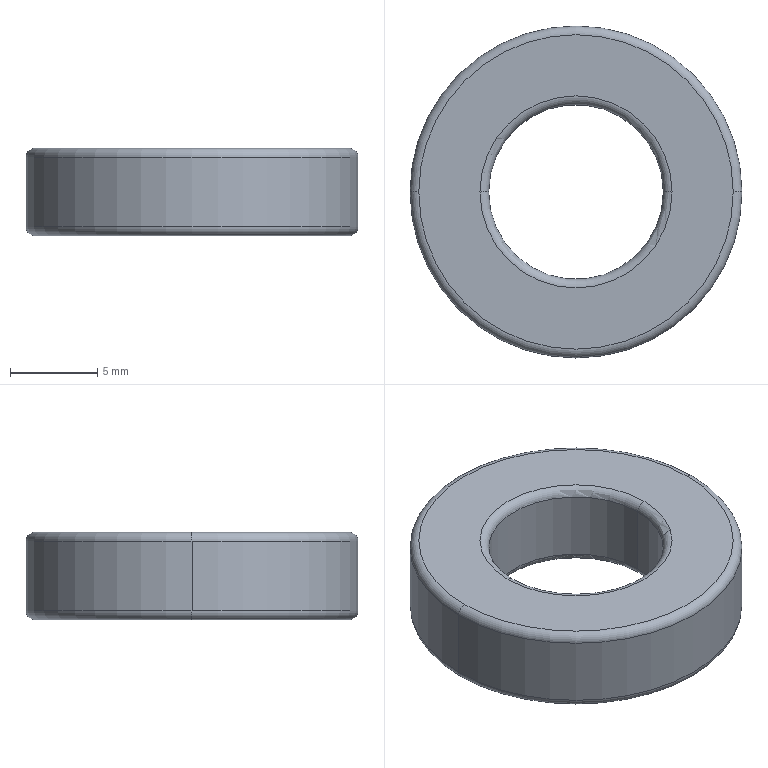Part | STEP file | 6800ZZ | 1 solid | 14 faces | box 19 x 19 x 5 mm | volume 1015 mm3 | torus 8 | cylinder 4 | plane 2 | commonest cylinder face diameters 10 x2 19 x2
STEP:
#1=CARTESIAN_POINT('',(0.,0.,0.));
#2=DIRECTION('',(0.,0.,1.));
#3=DIRECTION('',(1.,0.,0.));
#4=AXIS2_PLACEMENT_3D('',#1,#2,#3);
#5=CARTESIAN_POINT('',(-5.,0.,0.5));
#6=VERTEX_POINT('',#5);
#7=CARTESIAN_POINT('',(5.,0.,0.5));
#8=VERTEX_POINT('',#7);
#9=CARTESIAN_POINT('',(0.,0.,0.5));
#10=DIRECTION('',(0.,0.,-1.));
#11=DIRECTION('',(1.,0.,0.));
#12=AXIS2_PLACEMENT_3D('',#9,#10,#11);
#13=CIRCLE('',#12,5.);
#14=CARTESIAN_POINT('',(0.,0.,0.5));
#15=DIRECTION('',(0.,0.,1.));
#16=DIRECTION('',(1.,0.,0.));
#17=AXIS2_PLACEMENT_3D('',#14,#15,#16);
#18=TOROIDAL_SURFACE('',#17,5.5,0.5);
#19=CARTESIAN_POINT('',(6.283,3.142));
#20=DIRECTION('',(-1.,0.));
#21=VECTOR('',#20,1.);
#22=LINE('',#19,#21);
#23=(GEOMETRIC_REPRESENTATION_CONTEXT(2)PARAMETRIC_REPRESENTATION_CONTEXT()REPRESENTATION_CONTEXT('',''));
#24=DEFINITIONAL_REPRESENTATION('',(#22),#23);
#25=PCURVE('',#18,#24);
#26=CARTESIAN_POINT('',(0.,0.,5.));
#27=DIRECTION('',(0.,0.,-1.));
#28=DIRECTION('',(-1.,0.,0.));
#29=AXIS2_PLACEMENT_3D('',#26,#27,#28);
#30=CYLINDRICAL_SURFACE('',#29,5.);
#31=CARTESIAN_POINT('',(-3.142,4.5));
#32=DIRECTION('',(1.,0.));
#33=VECTOR('',#32,1.);
#34=LINE('',#31,#33);
#35=(GEOMETRIC_REPRESENTATION_CONTEXT(2)PARAMETRIC_REPRESENTATION_CONTEXT()REPRESENTATION_CONTEXT('',''));
#36=DEFINITIONAL_REPRESENTATION('',(#34),#35);
#37=PCURVE('',#30,#36);
#38=SURFACE_CURVE('',#13,(#25,#37),.PCURVE_S1.);
#39=EDGE_CURVE('',#6,#8,#38,.T.);
#40=ORIENTED_EDGE('',*,*,#39,.F.);
#41=CARTESIAN_POINT('',(-5.5,0.,0.));
#42=VERTEX_POINT('',#41);
#43=CARTESIAN_POINT('',(-5.5,0.,0.5));
#44=DIRECTION('',(0.,1.,0.));
#45=DIRECTION('',(-1.,0.,0.));
#46=AXIS2_PLACEMENT_3D('',#43,#44,#45);
#47=CIRCLE('',#46,0.5);
#48=CARTESIAN_POINT('',(3.142,0.));
#49=DIRECTION('',(0.,1.));
#50=VECTOR('',#49,1.);
#51=LINE('',#48,#50);
#52=(GEOMETRIC_REPRESENTATION_CONTEXT(2)PARAMETRIC_REPRESENTATION_CONTEXT()REPRESENTATION_CONTEXT('',''));
#53=DEFINITIONAL_REPRESENTATION('',(#51),#52);
#54=PCURVE('',#18,#53);
#55=CARTESIAN_POINT('',(0.,0.,0.5));
#56=DIRECTION('',(0.,0.,1.));
#57=DIRECTION('',(1.,0.,0.));
#58=AXIS2_PLACEMENT_3D('',#55,#56,#57);
#59=TOROIDAL_SURFACE('',#58,5.5,0.5);
#60=CARTESIAN_POINT('',(3.142,0.));
#61=DIRECTION('',(0.,1.));
#62=VECTOR('',#61,1.);
#63=LINE('',#60,#62);
#64=(GEOMETRIC_REPRESENTATION_CONTEXT(2)PARAMETRIC_REPRESENTATION_CONTEXT()REPRESENTATION_CONTEXT('',''));
#65=DEFINITIONAL_REPRESENTATION('',(#63),#64);
#66=PCURVE('',#59,#65);
#67=SURFACE_CURVE('',#47,(#54,#66),.PCURVE_S1.);
#68=EDGE_CURVE('',#6,#42,#67,.T.);
#69=ORIENTED_EDGE('',*,*,#68,.T.);
#70=CARTESIAN_POINT('',(5.5,0.,0.));
#71=VERTEX_POINT('',#70);
#72=CARTESIAN_POINT('',(0.,0.,0.));
#73=DIRECTION('',(0.,0.,1.));
#74=DIRECTION('',(1.,0.,0.));
#75=AXIS2_PLACEMENT_3D('',#72,#73,#74);
#76=CIRCLE('',#75,5.5);
#77=CARTESIAN_POINT('',(0.,4.712));
#78=DIRECTION('',(1.,0.));
#79=VECTOR('',#78,1.);
#80=LINE('',#77,#79);
#81=(GEOMETRIC_REPRESENTATION_CONTEXT(2)PARAMETRIC_REPRESENTATION_CONTEXT()REPRESENTATION_CONTEXT('',''));
#82=DEFINITIONAL_REPRESENTATION('',(#80),#81);
#83=PCURVE('',#18,#82);
#84=CARTESIAN_POINT('',(0.,0.,0.));
#85=DIRECTION('',(0.,0.,1.));
#86=DIRECTION('',(1.,0.,0.));
#87=AXIS2_PLACEMENT_3D('',#84,#85,#86);
#88=PLANE('',#87);
#89=CARTESIAN_POINT('',(0.,0.));
#90=DIRECTION('',(1.,0.));
#91=AXIS2_PLACEMENT_2D('',#89,#90);
#92=CIRCLE('',#91,5.5);
#93=(GEOMETRIC_REPRESENTATION_CONTEXT(2)PARAMETRIC_REPRESENTATION_CONTEXT()REPRESENTATION_CONTEXT('',''));
#94=DEFINITIONAL_REPRESENTATION('',(#92),#93);
#95=PCURVE('',#88,#94);
#96=SURFACE_CURVE('',#76,(#83,#95),.PCURVE_S1.);
#97=EDGE_CURVE('',#71,#42,#96,.T.);
#98=ORIENTED_EDGE('',*,*,#97,.F.);
#99=CARTESIAN_POINT('',(5.5,0.,0.5));
#100=DIRECTION('',(0.,-1.,0.));
#101=DIRECTION('',(0.,0.,-1.));
#102=AXIS2_PLACEMENT_3D('',#99,#100,#101);
#103=CIRCLE('',#102,0.5);
#104=CARTESIAN_POINT('',(0.,-1.571));
#105=DIRECTION('',(0.,1.));
#106=VECTOR('',#105,1.);
#107=LINE('',#104,#106);
#108=(GEOMETRIC_REPRESENTATION_CONTEXT(2)PARAMETRIC_REPRESENTATION_CONTEXT()REPRESENTATION_CONTEXT('',''));
#109=DEFINITIONAL_REPRESENTATION('',(#107),#108);
#110=PCURVE('',#18,#109);
#111=CARTESIAN_POINT('',(6.283,-1.571));
#112=DIRECTION('',(0.,1.));
#113=VECTOR('',#112,1.);
#114=LINE('',#111,#113);
#115=(GEOMETRIC_REPRESENTATION_CONTEXT(2)PARAMETRIC_REPRESENTATION_CONTEXT()REPRESENTATION_CONTEXT('',''));
#116=DEFINITIONAL_REPRESENTATION('',(#114),#115);
#117=PCURVE('',#59,#116);
#118=SURFACE_CURVE('',#103,(#110,#117),.PCURVE_S1.);
#119=EDGE_CURVE('',#8,#71,#118,.T.);
#120=ORIENTED_EDGE('',*,*,#119,.F.);
#121=EDGE_LOOP('',(#40,#69,#98,#120));
#122=FACE_BOUND('',#121,.T.);
#123=ADVANCED_FACE('',(#122),#18,.T.);
#124=CARTESIAN_POINT('',(-5.5,0.,5.));
#125=VERTEX_POINT('',#124);
#126=CARTESIAN_POINT('',(5.5,0.,5.));
#127=VERTEX_POINT('',#126);
#128=CARTESIAN_POINT('',(0.,0.,5.));
#129=DIRECTION('',(0.,0.,-1.));
#130=DIRECTION('',(1.,0.,0.));
#131=AXIS2_PLACEMENT_3D('',#128,#129,#130);
#132=CIRCLE('',#131,5.5);
#133=CARTESIAN_POINT('',(0.,0.,4.5));
#134=DIRECTION('',(0.,0.,1.));
#135=DIRECTION('',(1.,0.,0.));
#136=AXIS2_PLACEMENT_3D('',#133,#134,#135);
#137=TOROIDAL_SURFACE('',#136,5.5,0.5);
#138=CARTESIAN_POINT('',(6.283,1.571));
#139=DIRECTION('',(-1.,0.));
#140=VECTOR('',#139,1.);
#141=LINE('',#138,#140);
#142=(GEOMETRIC_REPRESENTATION_CONTEXT(2)PARAMETRIC_REPRESENTATION_CONTEXT()REPRESENTATION_CONTEXT('',''));
#143=DEFINITIONAL_REPRESENTATION('',(#141),#142);
#144=PCURVE('',#137,#143);
#145=CARTESIAN_POINT('',(0.,0.,5.));
#146=DIRECTION('',(0.,0.,1.));
#147=DIRECTION('',(1.,0.,0.));
#148=AXIS2_PLACEMENT_3D('',#145,#146,#147);
#149=PLANE('',#148);
#150=CARTESIAN_POINT('',(5.5,0.));
#151=CARTESIAN_POINT('',(5.5,-9.526));
#152=CARTESIAN_POINT('',(-2.75,-4.763));
#153=CARTESIAN_POINT('',(-11.,0.));
#154=CARTESIAN_POINT('',(-2.75,4.763));
#155=CARTESIAN_POINT('',(5.5,9.526));
#156=CARTESIAN_POINT('',(5.5,0.));
#157=(BOUNDED_CURVE()B_SPLINE_CURVE(2,(#150,#151,#152,#153,#154,#155,#156),.UNSPECIFIED.,.T.,.F.)B_SPLINE_CURVE_WITH_KNOTS((1,2,2,2,2,1),(-2.094,0.,2.094,4.189,6.283,8.378),.UNSPECIFIED.)CURVE()GEOMETRIC_REPRESENTATION_ITEM()RATIONAL_B_SPLINE_CURVE((1.,0.5,1.,0.5,1.,0.5,1.))REPRESENTATION_ITEM(''));
#158=(GEOMETRIC_REPRESENTATION_CONTEXT(2)PARAMETRIC_REPRESENTATION_CONTEXT()REPRESENTATION_CONTEXT('',''));
#159=DEFINITIONAL_REPRESENTATION('',(#157),#158);
#160=PCURVE('',#149,#159);
#161=SURFACE_CURVE('',#132,(#144,#160),.PCURVE_S1.);
#162=EDGE_CURVE('',#125,#127,#161,.T.);
#163=ORIENTED_EDGE('',*,*,#162,.F.);
#164=CARTESIAN_POINT('',(-5.,0.,4.5));
#165=VERTEX_POINT('',#164);
#166=CARTESIAN_POINT('',(-5.5,0.,4.5));
#167=DIRECTION('',(0.,1.,0.));
#168=DIRECTION('',(-1.,0.,0.));
#169=AXIS2_PLACEMENT_3D('',#166,#167,#168);
#170=CIRCLE('',#169,0.5);
#171=CARTESIAN_POINT('',(3.142,0.));
#172=DIRECTION('',(0.,1.));
#173=VECTOR('',#172,1.);
#174=LINE('',#171,#173);
#175=(GEOMETRIC_REPRESENTATION_CONTEXT(2)PARAMETRIC_REPRESENTATION_CONTEXT()REPRESENTATION_CONTEXT('',''));
#176=DEFINITIONAL_REPRESENTATION('',(#174),#175);
#177=PCURVE('',#137,#176);
#178=CARTESIAN_POINT('',(0.,0.,4.5));
#179=DIRECTION('',(0.,0.,1.));
#180=DIRECTION('',(1.,0.,0.));
#181=AXIS2_PLACEMENT_3D('',#178,#179,#180);
#182=TOROIDAL_SURFACE('',#181,5.5,0.5);
#183=CARTESIAN_POINT('',(3.142,0.));
#184=DIRECTION('',(0.,1.));
#185=VECTOR('',#184,1.);
#186=LINE('',#183,#185);
#187=(GEOMETRIC_REPRESENTATION_CONTEXT(2)PARAMETRIC_REPRESENTATION_CONTEXT()REPRESENTATION_CONTEXT('',''));
#188=DEFINITIONAL_REPRESENTATION('',(#186),#187);
#189=PCURVE('',#182,#188);
#190=SURFACE_CURVE('',#170,(#177,#189),.PCURVE_S1.);
#191=EDGE_CURVE('',#125,#165,#190,.T.);
#192=ORIENTED_EDGE('',*,*,#191,.T.);
#193=CARTESIAN_POINT('',(5.,0.,4.5));
#194=VERTEX_POINT('',#193);
#195=CARTESIAN_POINT('',(0.,0.,4.5));
#196=DIRECTION('',(0.,0.,1.));
#197=DIRECTION('',(1.,0.,0.));
#198=AXIS2_PLACEMENT_3D('',#195,#196,#197);
#199=CIRCLE('',#198,5.);
#200=CARTESIAN_POINT('',(0.,3.142));
#201=DIRECTION('',(1.,0.));
#202=VECTOR('',#201,1.);
#203=LINE('',#200,#202);
#204=(GEOMETRIC_REPRESENTATION_CONTEXT(2)PARAMETRIC_REPRESENTATION_CONTEXT()REPRESENTATION_CONTEXT('',''));
#205=DEFINITIONAL_REPRESENTATION('',(#203),#204);
#206=PCURVE('',#137,#205);
#207=CARTESIAN_POINT('',(3.142,0.5));
#208=DIRECTION('',(-1.,0.));
#209=VECTOR('',#208,1.);
#210=LINE('',#207,#209);
#211=(GEOMETRIC_REPRESENTATION_CONTEXT(2)PARAMETRIC_REPRESENTATION_CONTEXT()REPRESENTATION_CONTEXT('',''));
#212=DEFINITIONAL_REPRESENTATION('',(#210),#211);
#213=PCURVE('',#30,#212);
#214=SURFACE_CURVE('',#199,(#206,#213),.PCURVE_S1.);
#215=EDGE_CURVE('',#194,#165,#214,.T.);
#216=ORIENTED_EDGE('',*,*,#215,.F.);
#217=CARTESIAN_POINT('',(5.5,0.,4.5));
#218=DIRECTION('',(0.,-1.,0.));
#219=DIRECTION('',(0.,0.,-1.));
#220=AXIS2_PLACEMENT_3D('',#217,#218,#219);
#221=CIRCLE('',#220,0.5);
#222=CARTESIAN_POINT('',(0.,-1.571));
#223=DIRECTION('',(0.,1.));
#224=VECTOR('',#223,1.);
#225=LINE('',#222,#224);
#226=(GEOMETRIC_REPRESENTATION_CONTEXT(2)PARAMETRIC_REPRESENTATION_CONTEXT()REPRESENTATION_CONTEXT('',''));
#227=DEFINITIONAL_REPRESENTATION('',(#225),#226);
#228=PCURVE('',#137,#227);
#229=CARTESIAN_POINT('',(6.283,-1.571));
#230=DIRECTION('',(0.,1.));
#231=VECTOR('',#230,1.);
#232=LINE('',#229,#231);
#233=(GEOMETRIC_REPRESENTATION_CONTEXT(2)PARAMETRIC_REPRESENTATION_CONTEXT()REPRESENTATION_CONTEXT('',''));
#234=DEFINITIONAL_REPRESENTATION('',(#232),#233);
#235=PCURVE('',#182,#234);
#236=SURFACE_CURVE('',#221,(#228,#235),.PCURVE_S1.);
#237=EDGE_CURVE('',#127,#194,#236,.T.);
#238=ORIENTED_EDGE('',*,*,#237,.F.);
#239=EDGE_LOOP('',(#163,#192,#216,#238));
#240=FACE_BOUND('',#239,.T.);
#241=ADVANCED_FACE('',(#240),#137,.T.);
#242=CARTESIAN_POINT('',(-9.5,0.,4.5));
#243=VERTEX_POINT('',#242);
#244=CARTESIAN_POINT('',(9.5,0.,4.5));
#245=VERTEX_POINT('',#244);
#246=CARTESIAN_POINT('',(0.,0.,4.5));
#247=DIRECTION('',(0.,0.,-1.));
#248=DIRECTION('',(1.,0.,0.));
#249=AXIS2_PLACEMENT_3D('',#246,#247,#248);
#250=CIRCLE('',#249,9.5);
#251=CARTESIAN_POINT('',(0.,0.,4.5));
#252=DIRECTION('',(0.,0.,1.));
#253=DIRECTION('',(1.,0.,0.));
#254=AXIS2_PLACEMENT_3D('',#251,#252,#253);
#255=TOROIDAL_SURFACE('',#254,9.,0.5);
#256=CARTESIAN_POINT('',(6.283,0.));
#257=DIRECTION('',(-1.,0.));
#258=VECTOR('',#257,1.);
#259=LINE('',#256,#258);
#260=(GEOMETRIC_REPRESENTATION_CONTEXT(2)PARAMETRIC_REPRESENTATION_CONTEXT()REPRESENTATION_CONTEXT('',''));
#261=DEFINITIONAL_REPRESENTATION('',(#259),#260);
#262=PCURVE('',#255,#261);
#263=CARTESIAN_POINT('',(0.,0.,5.));
#264=DIRECTION('',(0.,0.,-1.));
#265=DIRECTION('',(-1.,0.,0.));
#266=AXIS2_PLACEMENT_3D('',#263,#264,#265);
#267=CYLINDRICAL_SURFACE('',#266,9.5);
#268=CARTESIAN_POINT('',(-3.142,0.5));
#269=DIRECTION('',(1.,0.));
#270=VECTOR('',#269,1.);
#271=LINE('',#268,#270);
#272=(GEOMETRIC_REPRESENTATION_CONTEXT(2)PARAMETRIC_REPRESENTATION_CONTEXT()REPRESENTATION_CONTEXT('',''));
#273=DEFINITIONAL_REPRESENTATION('',(#271),#272);
#274=PCURVE('',#267,#273);
#275=SURFACE_CURVE('',#250,(#262,#274),.PCURVE_S1.);
#276=EDGE_CURVE('',#243,#245,#275,.T.);
#277=ORIENTED_EDGE('',*,*,#276,.F.);
#278=CARTESIAN_POINT('',(-9.,0.,5.));
#279=VERTEX_POINT('',#278);
#280=CARTESIAN_POINT('',(-9.,0.,4.5));
#281=DIRECTION('',(0.,1.,0.));
#282=DIRECTION('',(-1.,0.,0.));
#283=AXIS2_PLACEMENT_3D('',#280,#281,#282);
#284=CIRCLE('',#283,0.5);
#285=CARTESIAN_POINT('',(3.142,0.));
#286=DIRECTION('',(0.,1.));
#287=VECTOR('',#286,1.);
#288=LINE('',#285,#287);
#289=(GEOMETRIC_REPRESENTATION_CONTEXT(2)PARAMETRIC_REPRESENTATION_CONTEXT()REPRESENTATION_CONTEXT('',''));
#290=DEFINITIONAL_REPRESENTATION('',(#288),#289);
#291=PCURVE('',#255,#290);
#292=CARTESIAN_POINT('',(0.,0.,4.5));
#293=DIRECTION('',(0.,0.,1.));
#294=DIRECTION('',(1.,0.,0.));
#295=AXIS2_PLACEMENT_3D('',#292,#293,#294);
#296=TOROIDAL_SURFACE('',#295,9.,0.5);
#297=CARTESIAN_POINT('',(3.142,0.));
#298=DIRECTION('',(0.,1.));
#299=VECTOR('',#298,1.);
#300=LINE('',#297,#299);
#301=(GEOMETRIC_REPRESENTATION_CONTEXT(2)PARAMETRIC_REPRESENTATION_CONTEXT()REPRESENTATION_CONTEXT('',''));
#302=DEFINITIONAL_REPRESENTATION('',(#300),#301);
#303=PCURVE('',#296,#302);
#304=SURFACE_CURVE('',#284,(#291,#303),.PCURVE_S1.);
#305=EDGE_CURVE('',#243,#279,#304,.T.);
#306=ORIENTED_EDGE('',*,*,#305,.T.);
#307=CARTESIAN_POINT('',(9.,0.,5.));
#308=VERTEX_POINT('',#307);
#309=CARTESIAN_POINT('',(0.,0.,5.));
#310=DIRECTION('',(0.,0.,1.));
#311=DIRECTION('',(1.,0.,0.));
#312=AXIS2_PLACEMENT_3D('',#309,#310,#311);
#313=CIRCLE('',#312,9.);
#314=CARTESIAN_POINT('',(0.,1.571));
#315=DIRECTION('',(1.,0.));
#316=VECTOR('',#315,1.);
#317=LINE('',#314,#316);
#318=(GEOMETRIC_REPRESENTATION_CONTEXT(2)PARAMETRIC_REPRESENTATION_CONTEXT()REPRESENTATION_CONTEXT('',''));
#319=DEFINITIONAL_REPRESENTATION('',(#317),#318);
#320=PCURVE('',#255,#319);
#321=CARTESIAN_POINT('',(0.,0.));
#322=DIRECTION('',(1.,0.));
#323=AXIS2_PLACEMENT_2D('',#321,#322);
#324=CIRCLE('',#323,9.);
#325=(GEOMETRIC_REPRESENTATION_CONTEXT(2)PARAMETRIC_REPRESENTATION_CONTEXT()REPRESENTATION_CONTEXT('',''));
#326=DEFINITIONAL_REPRESENTATION('',(#324),#325);
#327=PCURVE('',#149,#326);
#328=SURFACE_CURVE('',#313,(#320,#327),.PCURVE_S1.);
#329=EDGE_CURVE('',#308,#279,#328,.T.);
#330=ORIENTED_EDGE('',*,*,#329,.F.);
#331=CARTESIAN_POINT('',(9.,0.,4.5));
#332=DIRECTION('',(0.,-1.,0.));
#333=DIRECTION('',(0.,0.,-1.));
#334=AXIS2_PLACEMENT_3D('',#331,#332,#333);
#335=CIRCLE('',#334,0.5);
#336=CARTESIAN_POINT('',(0.,-1.571));
#337=DIRECTION('',(0.,1.));
#338=VECTOR('',#337,1.);
#339=LINE('',#336,#338);
#340=(GEOMETRIC_REPRESENTATION_CONTEXT(2)PARAMETRIC_REPRESENTATION_CONTEXT()REPRESENTATION_CONTEXT('',''));
#341=DEFINITIONAL_REPRESENTATION('',(#339),#340);
#342=PCURVE('',#255,#341);
#343=CARTESIAN_POINT('',(6.283,-1.571));
#344=DIRECTION('',(0.,1.));
#345=VECTOR('',#344,1.);
#346=LINE('',#343,#345);
#347=(GEOMETRIC_REPRESENTATION_CONTEXT(2)PARAMETRIC_REPRESENTATION_CONTEXT()REPRESENTATION_CONTEXT('',''));
#348=DEFINITIONAL_REPRESENTATION('',(#346),#347);
#349=PCURVE('',#296,#348);
#350=SURFACE_CURVE('',#335,(#342,#349),.PCURVE_S1.);
#351=EDGE_CURVE('',#245,#308,#350,.T.);
#352=ORIENTED_EDGE('',*,*,#351,.F.);
#353=EDGE_LOOP('',(#277,#306,#330,#352));
#354=FACE_BOUND('',#353,.T.);
#355=ADVANCED_FACE('',(#354),#255,.T.);
#356=CARTESIAN_POINT('',(-9.,0.,0.));
#357=VERTEX_POINT('',#356);
#358=CARTESIAN_POINT('',(9.,0.,0.));
#359=VERTEX_POINT('',#358);
#360=CARTESIAN_POINT('',(0.,0.,0.));
#361=DIRECTION('',(0.,0.,-1.));
#362=DIRECTION('',(1.,0.,0.));
#363=AXIS2_PLACEMENT_3D('',#360,#361,#362);
#364=CIRCLE('',#363,9.);
#365=CARTESIAN_POINT('',(0.,0.,0.5));
#366=DIRECTION('',(0.,0.,1.));
#367=DIRECTION('',(1.,0.,0.));
#368=AXIS2_PLACEMENT_3D('',#365,#366,#367);
#369=TOROIDAL_SURFACE('',#368,9.,0.5);
#370=CARTESIAN_POINT('',(6.283,4.712));
#371=DIRECTION('',(-1.,0.));
#372=VECTOR('',#371,1.);
#373=LINE('',#370,#372);
#374=(GEOMETRIC_REPRESENTATION_CONTEXT(2)PARAMETRIC_REPRESENTATION_CONTEXT()REPRESENTATION_CONTEXT('',''));
#375=DEFINITIONAL_REPRESENTATION('',(#373),#374);
#376=PCURVE('',#369,#375);
#377=CARTESIAN_POINT('',(9.,0.));
#378=CARTESIAN_POINT('',(9.,-15.588));
#379=CARTESIAN_POINT('',(-4.5,-7.794));
#380=CARTESIAN_POINT('',(-18.,0.));
#381=CARTESIAN_POINT('',(-4.5,7.794));
#382=CARTESIAN_POINT('',(9.,15.588));
#383=CARTESIAN_POINT('',(9.,0.));
#384=(BOUNDED_CURVE()B_SPLINE_CURVE(2,(#377,#378,#379,#380,#381,#382,#383),.UNSPECIFIED.,.T.,.F.)B_SPLINE_CURVE_WITH_KNOTS((1,2,2,2,2,1),(-2.094,0.,2.094,4.189,6.283,8.378),.UNSPECIFIED.)CURVE()GEOMETRIC_REPRESENTATION_ITEM()RATIONAL_B_SPLINE_CURVE((1.,0.5,1.,0.5,1.,0.5,1.))REPRESENTATION_ITEM(''));
#385=(GEOMETRIC_REPRESENTATION_CONTEXT(2)PARAMETRIC_REPRESENTATION_CONTEXT()REPRESENTATION_CONTEXT('',''));
#386=DEFINITIONAL_REPRESENTATION('',(#384),#385);
#387=PCURVE('',#88,#386);
#388=SURFACE_CURVE('',#364,(#376,#387),.PCURVE_S1.);
#389=EDGE_CURVE('',#357,#359,#388,.T.);
#390=ORIENTED_EDGE('',*,*,#389,.F.);
#391=CARTESIAN_POINT('',(-9.5,0.,0.5));
#392=VERTEX_POINT('',#391);
#393=CARTESIAN_POINT('',(-9.,0.,0.5));
#394=DIRECTION('',(0.,1.,0.));
#395=DIRECTION('',(-1.,0.,0.));
#396=AXIS2_PLACEMENT_3D('',#393,#394,#395);
#397=CIRCLE('',#396,0.5);
#398=CARTESIAN_POINT('',(3.142,0.));
#399=DIRECTION('',(0.,1.));
#400=VECTOR('',#399,1.);
#401=LINE('',#398,#400);
#402=(GEOMETRIC_REPRESENTATION_CONTEXT(2)PARAMETRIC_REPRESENTATION_CONTEXT()REPRESENTATION_CONTEXT('',''));
#403=DEFINITIONAL_REPRESENTATION('',(#401),#402);
#404=PCURVE('',#369,#403);
#405=CARTESIAN_POINT('',(0.,0.,0.5));
#406=DIRECTION('',(0.,0.,1.));
#407=DIRECTION('',(1.,0.,0.));
#408=AXIS2_PLACEMENT_3D('',#405,#406,#407);
#409=TOROIDAL_SURFACE('',#408,9.,0.5);
#410=CARTESIAN_POINT('',(3.142,0.));
#411=DIRECTION('',(0.,1.));
#412=VECTOR('',#411,1.);
#413=LINE('',#410,#412);
#414=(GEOMETRIC_REPRESENTATION_CONTEXT(2)PARAMETRIC_REPRESENTATION_CONTEXT()REPRESENTATION_CONTEXT('',''));
#415=DEFINITIONAL_REPRESENTATION('',(#413),#414);
#416=PCURVE('',#409,#415);
#417=SURFACE_CURVE('',#397,(#404,#416),.PCURVE_S1.);
#418=EDGE_CURVE('',#357,#392,#417,.T.);
#419=ORIENTED_EDGE('',*,*,#418,.T.);
#420=CARTESIAN_POINT('',(9.5,0.,0.5));
#421=VERTEX_POINT('',#420);
#422=CARTESIAN_POINT('',(0.,0.,0.5));
#423=DIRECTION('',(0.,0.,1.));
#424=DIRECTION('',(1.,0.,0.));
#425=AXIS2_PLACEMENT_3D('',#422,#423,#424);
#426=CIRCLE('',#425,9.5);
#427=CARTESIAN_POINT('',(0.,6.283));
#428=DIRECTION('',(1.,0.));
#429=VECTOR('',#428,1.);
#430=LINE('',#427,#429);
#431=(GEOMETRIC_REPRESENTATION_CONTEXT(2)PARAMETRIC_REPRESENTATION_CONTEXT()REPRESENTATION_CONTEXT('',''));
#432=DEFINITIONAL_REPRESENTATION('',(#430),#431);
#433=PCURVE('',#369,#432);
#434=CARTESIAN_POINT('',(3.142,4.5));
#435=DIRECTION('',(-1.,0.));
#436=VECTOR('',#435,1.);
#437=LINE('',#434,#436);
#438=(GEOMETRIC_REPRESENTATION_CONTEXT(2)PARAMETRIC_REPRESENTATION_CONTEXT()REPRESENTATION_CONTEXT('',''));
#439=DEFINITIONAL_REPRESENTATION('',(#437),#438);
#440=PCURVE('',#267,#439);
#441=SURFACE_CURVE('',#426,(#433,#440),.PCURVE_S1.);
#442=EDGE_CURVE('',#421,#392,#441,.T.);
#443=ORIENTED_EDGE('',*,*,#442,.F.);
#444=CARTESIAN_POINT('',(9.,0.,0.5));
#445=DIRECTION('',(0.,-1.,0.));
#446=DIRECTION('',(0.,0.,-1.));
#447=AXIS2_PLACEMENT_3D('',#444,#445,#446);
#448=CIRCLE('',#447,0.5);
#449=CARTESIAN_POINT('',(0.,4.712));
#450=DIRECTION('',(0.,1.));
#451=VECTOR('',#450,1.);
#452=LINE('',#449,#451);
#453=(GEOMETRIC_REPRESENTATION_CONTEXT(2)PARAMETRIC_REPRESENTATION_CONTEXT()REPRESENTATION_CONTEXT('',''));
#454=DEFINITIONAL_REPRESENTATION('',(#452),#453);
#455=PCURVE('',#369,#454);
#456=CARTESIAN_POINT('',(6.283,4.712));
#457=DIRECTION('',(0.,1.));
#458=VECTOR('',#457,1.);
#459=LINE('',#456,#458);
#460=(GEOMETRIC_REPRESENTATION_CONTEXT(2)PARAMETRIC_REPRESENTATION_CONTEXT()REPRESENTATION_CONTEXT('',''));
#461=DEFINITIONAL_REPRESENTATION('',(#459),#460);
#462=PCURVE('',#409,#461);
#463=SURFACE_CURVE('',#448,(#455,#462),.PCURVE_S1.);
#464=EDGE_CURVE('',#359,#421,#463,.T.);
#465=ORIENTED_EDGE('',*,*,#464,.F.);
#466=EDGE_LOOP('',(#390,#419,#443,#465));
#467=FACE_BOUND('',#466,.T.);
#468=ADVANCED_FACE('',(#467),#369,.T.);
#469=CARTESIAN_POINT('',(-5.,0.,5.));
#470=DIRECTION('',(0.,0.,-1.));
#471=VECTOR('',#470,1.);
#472=LINE('',#469,#471);
#473=CARTESIAN_POINT('',(0.,0.,5.));
#474=DIRECTION('',(0.,0.,-1.));
#475=DIRECTION('',(-1.,0.,0.));
#476=AXIS2_PLACEMENT_3D('',#473,#474,#475);
#477=CYLINDRICAL_SURFACE('',#476,5.);
#478=CARTESIAN_POINT('',(6.283,0.));
#479=DIRECTION('',(0.,1.));
#480=VECTOR('',#479,1.);
#481=LINE('',#478,#480);
#482=(GEOMETRIC_REPRESENTATION_CONTEXT(2)PARAMETRIC_REPRESENTATION_CONTEXT()REPRESENTATION_CONTEXT('',''));
#483=DEFINITIONAL_REPRESENTATION('',(#481),#482);
#484=PCURVE('',#477,#483);
#485=CARTESIAN_POINT('',(0.,0.));
#486=DIRECTION('',(0.,1.));
#487=VECTOR('',#486,1.);
#488=LINE('',#485,#487);
#489=(GEOMETRIC_REPRESENTATION_CONTEXT(2)PARAMETRIC_REPRESENTATION_CONTEXT()REPRESENTATION_CONTEXT('',''));
#490=DEFINITIONAL_REPRESENTATION('',(#488),#489);
#491=PCURVE('',#30,#490);
#492=SURFACE_CURVE('',#472,(#484,#491),.PCURVE_S1.);
#493=EDGE_CURVE('',#165,#6,#492,.T.);
#494=ORIENTED_EDGE('',*,*,#493,.T.);
#495=CARTESIAN_POINT('',(0.,0.,0.5));
#496=DIRECTION('',(0.,0.,-1.));
#497=DIRECTION('',(1.,0.,0.));
#498=AXIS2_PLACEMENT_3D('',#495,#496,#497);
#499=CIRCLE('',#498,5.);
#500=CARTESIAN_POINT('',(3.142,4.5));
#501=DIRECTION('',(1.,0.));
#502=VECTOR('',#501,1.);
#503=LINE('',#500,#502);
#504=(GEOMETRIC_REPRESENTATION_CONTEXT(2)PARAMETRIC_REPRESENTATION_CONTEXT()REPRESENTATION_CONTEXT('',''));
#505=DEFINITIONAL_REPRESENTATION('',(#503),#504);
#506=PCURVE('',#477,#505);
#507=CARTESIAN_POINT('',(6.283,3.142));
#508=DIRECTION('',(-1.,0.));
#509=VECTOR('',#508,1.);
#510=LINE('',#507,#509);
#511=(GEOMETRIC_REPRESENTATION_CONTEXT(2)PARAMETRIC_REPRESENTATION_CONTEXT()REPRESENTATION_CONTEXT('',''));
#512=DEFINITIONAL_REPRESENTATION('',(#510),#511);
#513=PCURVE('',#59,#512);
#514=SURFACE_CURVE('',#499,(#506,#513),.PCURVE_S1.);
#515=EDGE_CURVE('',#8,#6,#514,.T.);
#516=ORIENTED_EDGE('',*,*,#515,.F.);
#517=CARTESIAN_POINT('',(5.,0.,5.));
#518=DIRECTION('',(0.,0.,-1.));
#519=VECTOR('',#518,1.);
#520=LINE('',#517,#519);
#521=CARTESIAN_POINT('',(3.142,0.));
#522=DIRECTION('',(0.,1.));
#523=VECTOR('',#522,1.);
#524=LINE('',#521,#523);
#525=(GEOMETRIC_REPRESENTATION_CONTEXT(2)PARAMETRIC_REPRESENTATION_CONTEXT()REPRESENTATION_CONTEXT('',''));
#526=DEFINITIONAL_REPRESENTATION('',(#524),#525);
#527=PCURVE('',#477,#526);
#528=CARTESIAN_POINT('',(3.142,0.));
#529=DIRECTION('',(0.,1.));
#530=VECTOR('',#529,1.);
#531=LINE('',#528,#530);
#532=(GEOMETRIC_REPRESENTATION_CONTEXT(2)PARAMETRIC_REPRESENTATION_CONTEXT()REPRESENTATION_CONTEXT('',''));
#533=DEFINITIONAL_REPRESENTATION('',(#531),#532);
#534=PCURVE('',#30,#533);
#535=SURFACE_CURVE('',#520,(#527,#534),.PCURVE_S1.);
#536=EDGE_CURVE('',#194,#8,#535,.T.);
#537=ORIENTED_EDGE('',*,*,#536,.F.);
#538=CARTESIAN_POINT('',(0.,0.,4.5));
#539=DIRECTION('',(0.,0.,1.));
#540=DIRECTION('',(1.,0.,0.));
#541=AXIS2_PLACEMENT_3D('',#538,#539,#540);
#542=CIRCLE('',#541,5.);
#543=CARTESIAN_POINT('',(9.425,0.5));
#544=DIRECTION('',(-1.,0.));
#545=VECTOR('',#544,1.);
#546=LINE('',#543,#545);
#547=(GEOMETRIC_REPRESENTATION_CONTEXT(2)PARAMETRIC_REPRESENTATION_CONTEXT()REPRESENTATION_CONTEXT('',''));
#548=DEFINITIONAL_REPRESENTATION('',(#546),#547);
#549=PCURVE('',#477,#548);
#550=CARTESIAN_POINT('',(0.,3.142));
#551=DIRECTION('',(1.,0.));
#552=VECTOR('',#551,1.);
#553=LINE('',#550,#552);
#554=(GEOMETRIC_REPRESENTATION_CONTEXT(2)PARAMETRIC_REPRESENTATION_CONTEXT()REPRESENTATION_CONTEXT('',''));
#555=DEFINITIONAL_REPRESENTATION('',(#553),#554);
#556=PCURVE('',#182,#555);
#557=SURFACE_CURVE('',#542,(#549,#556),.PCURVE_S1.);
#558=EDGE_CURVE('',#165,#194,#557,.T.);
#559=ORIENTED_EDGE('',*,*,#558,.F.);
#560=EDGE_LOOP('',(#494,#516,#537,#559));
#561=FACE_BOUND('',#560,.F.);
#562=ADVANCED_FACE('',(#561),#477,.F.);
#563=ORIENTED_EDGE('',*,*,#276,.T.);
#564=CARTESIAN_POINT('',(9.5,0.,5.));
#565=DIRECTION('',(0.,0.,-1.));
#566=VECTOR('',#565,1.);
#567=LINE('',#564,#566);
#568=CARTESIAN_POINT('',(3.142,0.));
#569=DIRECTION('',(0.,1.));
#570=VECTOR('',#569,1.);
#571=LINE('',#568,#570);
#572=(GEOMETRIC_REPRESENTATION_CONTEXT(2)PARAMETRIC_REPRESENTATION_CONTEXT()REPRESENTATION_CONTEXT('',''));
#573=DEFINITIONAL_REPRESENTATION('',(#571),#572);
#574=PCURVE('',#267,#573);
#575=CARTESIAN_POINT('',(0.,0.,5.));
#576=DIRECTION('',(0.,0.,-1.));
#577=DIRECTION('',(-1.,0.,0.));
#578=AXIS2_PLACEMENT_3D('',#575,#576,#577);
#579=CYLINDRICAL_SURFACE('',#578,9.5);
#580=CARTESIAN_POINT('',(3.142,0.));
#581=DIRECTION('',(0.,1.));
#582=VECTOR('',#581,1.);
#583=LINE('',#580,#582);
#584=(GEOMETRIC_REPRESENTATION_CONTEXT(2)PARAMETRIC_REPRESENTATION_CONTEXT()REPRESENTATION_CONTEXT('',''));
#585=DEFINITIONAL_REPRESENTATION('',(#583),#584);
#586=PCURVE('',#579,#585);
#587=SURFACE_CURVE('',#567,(#574,#586),.PCURVE_S1.);
#588=EDGE_CURVE('',#245,#421,#587,.T.);
#589=ORIENTED_EDGE('',*,*,#588,.T.);
#590=ORIENTED_EDGE('',*,*,#442,.T.);
#591=CARTESIAN_POINT('',(-9.5,0.,5.));
#592=DIRECTION('',(0.,0.,-1.));
#593=VECTOR('',#592,1.);
#594=LINE('',#591,#593);
#595=CARTESIAN_POINT('',(0.,0.));
#596=DIRECTION('',(0.,1.));
#597=VECTOR('',#596,1.);
#598=LINE('',#595,#597);
#599=(GEOMETRIC_REPRESENTATION_CONTEXT(2)PARAMETRIC_REPRESENTATION_CONTEXT()REPRESENTATION_CONTEXT('',''));
#600=DEFINITIONAL_REPRESENTATION('',(#598),#599);
#601=PCURVE('',#267,#600);
#602=CARTESIAN_POINT('',(6.283,0.));
#603=DIRECTION('',(0.,1.));
#604=VECTOR('',#603,1.);
#605=LINE('',#602,#604);
#606=(GEOMETRIC_REPRESENTATION_CONTEXT(2)PARAMETRIC_REPRESENTATION_CONTEXT()REPRESENTATION_CONTEXT('',''));
#607=DEFINITIONAL_REPRESENTATION('',(#605),#606);
#608=PCURVE('',#579,#607);
#609=SURFACE_CURVE('',#594,(#601,#608),.PCURVE_S1.);
#610=EDGE_CURVE('',#243,#392,#609,.T.);
#611=ORIENTED_EDGE('',*,*,#610,.F.);
#612=EDGE_LOOP('',(#563,#589,#590,#611));
#613=FACE_BOUND('',#612,.T.);
#614=ADVANCED_FACE('',(#613),#267,.T.);
#615=ORIENTED_EDGE('',*,*,#329,.T.);
#616=CARTESIAN_POINT('',(0.,0.,5.));
#617=DIRECTION('',(0.,0.,1.));
#618=DIRECTION('',(1.,0.,0.));
#619=AXIS2_PLACEMENT_3D('',#616,#617,#618);
#620=CIRCLE('',#619,9.);
#621=CARTESIAN_POINT('',(0.,0.));
#622=DIRECTION('',(1.,0.));
#623=AXIS2_PLACEMENT_2D('',#621,#622);
#624=CIRCLE('',#623,9.);
#625=(GEOMETRIC_REPRESENTATION_CONTEXT(2)PARAMETRIC_REPRESENTATION_CONTEXT()REPRESENTATION_CONTEXT('',''));
#626=DEFINITIONAL_REPRESENTATION('',(#624),#625);
#627=PCURVE('',#149,#626);
#628=CARTESIAN_POINT('',(0.,1.571));
#629=DIRECTION('',(1.,0.));
#630=VECTOR('',#629,1.);
#631=LINE('',#628,#630);
#632=(GEOMETRIC_REPRESENTATION_CONTEXT(2)PARAMETRIC_REPRESENTATION_CONTEXT()REPRESENTATION_CONTEXT('',''));
#633=DEFINITIONAL_REPRESENTATION('',(#631),#632);
#634=PCURVE('',#296,#633);
#635=SURFACE_CURVE('',#620,(#627,#634),.PCURVE_S1.);
#636=EDGE_CURVE('',#279,#308,#635,.T.);
#637=ORIENTED_EDGE('',*,*,#636,.T.);
#638=EDGE_LOOP('',(#615,#637));
#639=FACE_BOUND('',#638,.T.);
#640=CARTESIAN_POINT('',(0.,0.,5.));
#641=DIRECTION('',(0.,0.,-1.));
#642=DIRECTION('',(1.,0.,0.));
#643=AXIS2_PLACEMENT_3D('',#640,#641,#642);
#644=CIRCLE('',#643,5.5);
#645=CARTESIAN_POINT('',(5.5,0.));
#646=CARTESIAN_POINT('',(5.5,-9.526));
#647=CARTESIAN_POINT('',(-2.75,-4.763));
#648=CARTESIAN_POINT('',(-11.,0.));
#649=CARTESIAN_POINT('',(-2.75,4.763));
#650=CARTESIAN_POINT('',(5.5,9.526));
#651=CARTESIAN_POINT('',(5.5,0.));
#652=(BOUNDED_CURVE()B_SPLINE_CURVE(2,(#645,#646,#647,#648,#649,#650,#651),.UNSPECIFIED.,.T.,.F.)B_SPLINE_CURVE_WITH_KNOTS((1,2,2,2,2,1),(-2.094,0.,2.094,4.189,6.283,8.378),.UNSPECIFIED.)CURVE()GEOMETRIC_REPRESENTATION_ITEM()RATIONAL_B_SPLINE_CURVE((1.,0.5,1.,0.5,1.,0.5,1.))REPRESENTATION_ITEM(''));
#653=(GEOMETRIC_REPRESENTATION_CONTEXT(2)PARAMETRIC_REPRESENTATION_CONTEXT()REPRESENTATION_CONTEXT('',''));
#654=DEFINITIONAL_REPRESENTATION('',(#652),#653);
#655=PCURVE('',#149,#654);
#656=CARTESIAN_POINT('',(6.283,1.571));
#657=DIRECTION('',(-1.,0.));
#658=VECTOR('',#657,1.);
#659=LINE('',#656,#658);
#660=(GEOMETRIC_REPRESENTATION_CONTEXT(2)PARAMETRIC_REPRESENTATION_CONTEXT()REPRESENTATION_CONTEXT('',''));
#661=DEFINITIONAL_REPRESENTATION('',(#659),#660);
#662=PCURVE('',#182,#661);
#663=SURFACE_CURVE('',#644,(#655,#662),.PCURVE_S1.);
#664=EDGE_CURVE('',#127,#125,#663,.T.);
#665=ORIENTED_EDGE('',*,*,#664,.T.);
#666=ORIENTED_EDGE('',*,*,#162,.T.);
#667=EDGE_LOOP('',(#665,#666));
#668=FACE_BOUND('',#667,.T.);
#669=ADVANCED_FACE('',(#639,#668),#149,.T.);
#670=CARTESIAN_POINT('',(0.,0.,0.));
#671=DIRECTION('',(0.,0.,-1.));
#672=DIRECTION('',(1.,0.,0.));
#673=AXIS2_PLACEMENT_3D('',#670,#671,#672);
#674=CIRCLE('',#673,9.);
#675=CARTESIAN_POINT('',(9.,0.));
#676=CARTESIAN_POINT('',(9.,-15.588));
#677=CARTESIAN_POINT('',(-4.5,-7.794));
#678=CARTESIAN_POINT('',(-18.,0.));
#679=CARTESIAN_POINT('',(-4.5,7.794));
#680=CARTESIAN_POINT('',(9.,15.588));
#681=CARTESIAN_POINT('',(9.,0.));
#682=(BOUNDED_CURVE()B_SPLINE_CURVE(2,(#675,#676,#677,#678,#679,#680,#681),.UNSPECIFIED.,.T.,.F.)B_SPLINE_CURVE_WITH_KNOTS((1,2,2,2,2,1),(-2.094,0.,2.094,4.189,6.283,8.378),.UNSPECIFIED.)CURVE()GEOMETRIC_REPRESENTATION_ITEM()RATIONAL_B_SPLINE_CURVE((1.,0.5,1.,0.5,1.,0.5,1.))REPRESENTATION_ITEM(''));
#683=(GEOMETRIC_REPRESENTATION_CONTEXT(2)PARAMETRIC_REPRESENTATION_CONTEXT()REPRESENTATION_CONTEXT('',''));
#684=DEFINITIONAL_REPRESENTATION('',(#682),#683);
#685=PCURVE('',#88,#684);
#686=CARTESIAN_POINT('',(6.283,4.712));
#687=DIRECTION('',(-1.,0.));
#688=VECTOR('',#687,1.);
#689=LINE('',#686,#688);
#690=(GEOMETRIC_REPRESENTATION_CONTEXT(2)PARAMETRIC_REPRESENTATION_CONTEXT()REPRESENTATION_CONTEXT('',''));
#691=DEFINITIONAL_REPRESENTATION('',(#689),#690);
#692=PCURVE('',#409,#691);
#693=SURFACE_CURVE('',#674,(#685,#692),.PCURVE_S1.);
#694=EDGE_CURVE('',#359,#357,#693,.T.);
#695=ORIENTED_EDGE('',*,*,#694,.T.);
#696=ORIENTED_EDGE('',*,*,#389,.T.);
#697=EDGE_LOOP('',(#695,#696));
#698=FACE_BOUND('',#697,.T.);
#699=ORIENTED_EDGE('',*,*,#97,.T.);
#700=CARTESIAN_POINT('',(0.,0.,0.));
#701=DIRECTION('',(0.,0.,1.));
#702=DIRECTION('',(1.,0.,0.));
#703=AXIS2_PLACEMENT_3D('',#700,#701,#702);
#704=CIRCLE('',#703,5.5);
#705=CARTESIAN_POINT('',(0.,0.));
#706=DIRECTION('',(1.,0.));
#707=AXIS2_PLACEMENT_2D('',#705,#706);
#708=CIRCLE('',#707,5.5);
#709=(GEOMETRIC_REPRESENTATION_CONTEXT(2)PARAMETRIC_REPRESENTATION_CONTEXT()REPRESENTATION_CONTEXT('',''));
#710=DEFINITIONAL_REPRESENTATION('',(#708),#709);
#711=PCURVE('',#88,#710);
#712=CARTESIAN_POINT('',(0.,4.712));
#713=DIRECTION('',(1.,0.));
#714=VECTOR('',#713,1.);
#715=LINE('',#712,#714);
#716=(GEOMETRIC_REPRESENTATION_CONTEXT(2)PARAMETRIC_REPRESENTATION_CONTEXT()REPRESENTATION_CONTEXT('',''));
#717=DEFINITIONAL_REPRESENTATION('',(#715),#716);
#718=PCURVE('',#59,#717);
#719=SURFACE_CURVE('',#704,(#711,#718),.PCURVE_S1.);
#720=EDGE_CURVE('',#42,#71,#719,.T.);
#721=ORIENTED_EDGE('',*,*,#720,.T.);
#722=EDGE_LOOP('',(#699,#721));
#723=FACE_BOUND('',#722,.T.);
#724=ADVANCED_FACE('',(#698,#723),#88,.F.);
#725=ORIENTED_EDGE('',*,*,#588,.F.);
#726=CARTESIAN_POINT('',(0.,0.,4.5));
#727=DIRECTION('',(0.,0.,-1.));
#728=DIRECTION('',(1.,0.,0.));
#729=AXIS2_PLACEMENT_3D('',#726,#727,#728);
#730=CIRCLE('',#729,9.5);
#731=CARTESIAN_POINT('',(3.142,0.5));
#732=DIRECTION('',(1.,0.));
#733=VECTOR('',#732,1.);
#734=LINE('',#731,#733);
#735=(GEOMETRIC_REPRESENTATION_CONTEXT(2)PARAMETRIC_REPRESENTATION_CONTEXT()REPRESENTATION_CONTEXT('',''));
#736=DEFINITIONAL_REPRESENTATION('',(#734),#735);
#737=PCURVE('',#579,#736);
#738=CARTESIAN_POINT('',(6.283,0.));
#739=DIRECTION('',(-1.,0.));
#740=VECTOR('',#739,1.);
#741=LINE('',#738,#740);
#742=(GEOMETRIC_REPRESENTATION_CONTEXT(2)PARAMETRIC_REPRESENTATION_CONTEXT()REPRESENTATION_CONTEXT('',''));
#743=DEFINITIONAL_REPRESENTATION('',(#741),#742);
#744=PCURVE('',#296,#743);
#745=SURFACE_CURVE('',#730,(#737,#744),.PCURVE_S1.);
#746=EDGE_CURVE('',#245,#243,#745,.T.);
#747=ORIENTED_EDGE('',*,*,#746,.T.);
#748=ORIENTED_EDGE('',*,*,#610,.T.);
#749=CARTESIAN_POINT('',(0.,0.,0.5));
#750=DIRECTION('',(0.,0.,1.));
#751=DIRECTION('',(1.,0.,0.));
#752=AXIS2_PLACEMENT_3D('',#749,#750,#751);
#753=CIRCLE('',#752,9.5);
#754=CARTESIAN_POINT('',(9.425,4.5));
#755=DIRECTION('',(-1.,0.));
#756=VECTOR('',#755,1.);
#757=LINE('',#754,#756);
#758=(GEOMETRIC_REPRESENTATION_CONTEXT(2)PARAMETRIC_REPRESENTATION_CONTEXT()REPRESENTATION_CONTEXT('',''));
#759=DEFINITIONAL_REPRESENTATION('',(#757),#758);
#760=PCURVE('',#579,#759);
#761=CARTESIAN_POINT('',(0.,6.283));
#762=DIRECTION('',(1.,0.));
#763=VECTOR('',#762,1.);
#764=LINE('',#761,#763);
#765=(GEOMETRIC_REPRESENTATION_CONTEXT(2)PARAMETRIC_REPRESENTATION_CONTEXT()REPRESENTATION_CONTEXT('',''));
#766=DEFINITIONAL_REPRESENTATION('',(#764),#765);
#767=PCURVE('',#409,#766);
#768=SURFACE_CURVE('',#753,(#760,#767),.PCURVE_S1.);
#769=EDGE_CURVE('',#392,#421,#768,.T.);
#770=ORIENTED_EDGE('',*,*,#769,.T.);
#771=EDGE_LOOP('',(#725,#747,#748,#770));
#772=FACE_BOUND('',#771,.T.);
#773=ADVANCED_FACE('',(#772),#579,.T.);
#774=ORIENTED_EDGE('',*,*,#39,.F.);
#775=ORIENTED_EDGE('',*,*,#493,.F.);
#776=ORIENTED_EDGE('',*,*,#215,.F.);
#777=ORIENTED_EDGE('',*,*,#536,.T.);
#778=EDGE_LOOP('',(#774,#775,#776,#777));
#779=FACE_BOUND('',#778,.F.);
#780=ADVANCED_FACE('',(#779),#30,.F.);
#781=ORIENTED_EDGE('',*,*,#418,.F.);
#782=ORIENTED_EDGE('',*,*,#694,.F.);
#783=ORIENTED_EDGE('',*,*,#464,.T.);
#784=ORIENTED_EDGE('',*,*,#769,.F.);
#785=EDGE_LOOP('',(#781,#782,#783,#784));
#786=FACE_BOUND('',#785,.T.);
#787=ADVANCED_FACE('',(#786),#409,.T.);
#788=ORIENTED_EDGE('',*,*,#305,.F.);
#789=ORIENTED_EDGE('',*,*,#746,.F.);
#790=ORIENTED_EDGE('',*,*,#351,.T.);
#791=ORIENTED_EDGE('',*,*,#636,.F.);
#792=EDGE_LOOP('',(#788,#789,#790,#791));
#793=FACE_BOUND('',#792,.T.);
#794=ADVANCED_FACE('',(#793),#296,.T.);
#795=ORIENTED_EDGE('',*,*,#191,.F.);
#796=ORIENTED_EDGE('',*,*,#664,.F.);
#797=ORIENTED_EDGE('',*,*,#237,.T.);
#798=ORIENTED_EDGE('',*,*,#558,.F.);
#799=EDGE_LOOP('',(#795,#796,#797,#798));
#800=FACE_BOUND('',#799,.T.);
#801=ADVANCED_FACE('',(#800),#182,.T.);
#802=ORIENTED_EDGE('',*,*,#68,.F.);
#803=ORIENTED_EDGE('',*,*,#515,.F.);
#804=ORIENTED_EDGE('',*,*,#119,.T.);
#805=ORIENTED_EDGE('',*,*,#720,.F.);
#806=EDGE_LOOP('',(#802,#803,#804,#805));
#807=FACE_BOUND('',#806,.T.);
#808=ADVANCED_FACE('',(#807),#59,.T.);
#809=CLOSED_SHELL('',(#123,#241,#355,#468,#562,#614,#669,#724,#773,#780,#787,#794,#801,#808));
#810=MANIFOLD_SOLID_BREP('',#809);
#811=(LENGTH_UNIT()NAMED_UNIT(*)SI_UNIT(.MILLI.,.METRE.));
#812=UNCERTAINTY_MEASURE_WITH_UNIT(LENGTH_MEASURE(0.0000001),#811,'','');
#813=(NAMED_UNIT(*)PLANE_ANGLE_UNIT()SI_UNIT($,.RADIAN.));
#814=(NAMED_UNIT(*)SI_UNIT($,.STERADIAN.)SOLID_ANGLE_UNIT());
#815=(GEOMETRIC_REPRESENTATION_CONTEXT(3)GLOBAL_UNCERTAINTY_ASSIGNED_CONTEXT((#812))GLOBAL_UNIT_ASSIGNED_CONTEXT((#811,#813,#814))REPRESENTATION_CONTEXT('',''));
#816=ADVANCED_BREP_SHAPE_REPRESENTATION('',(#4,#810),#815);